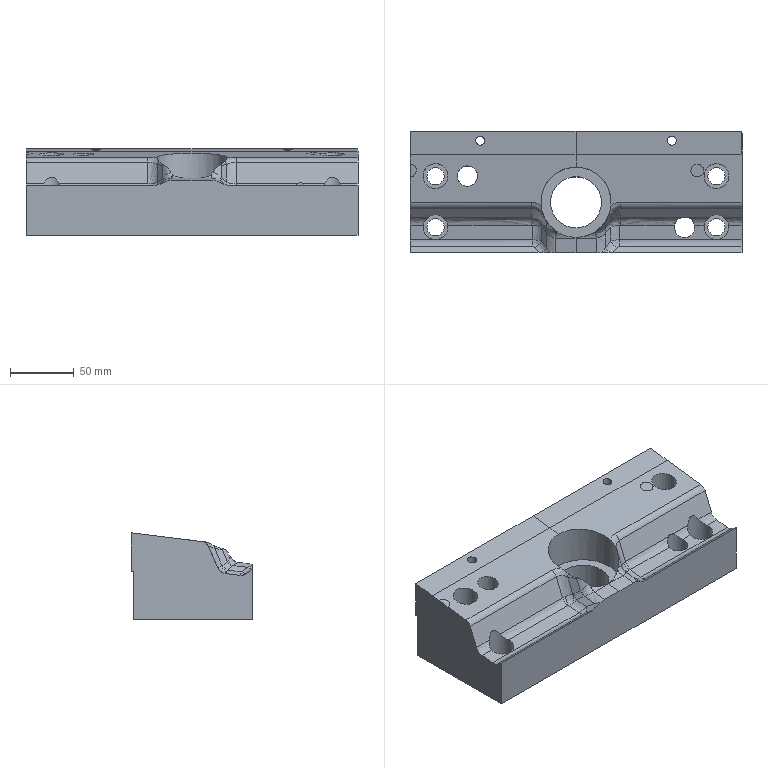Part | NX | features solid 2 | 1 solid | 98 faces | box 260 x 95.176 x 67.682 mm | volume 1170340 mm3 | spline 67 | cylinder 16 | plane 15 | commonest cylinder face diameters 13.5 x4 19.5 x4 7 x2 10 x2 16 x2 40 x1